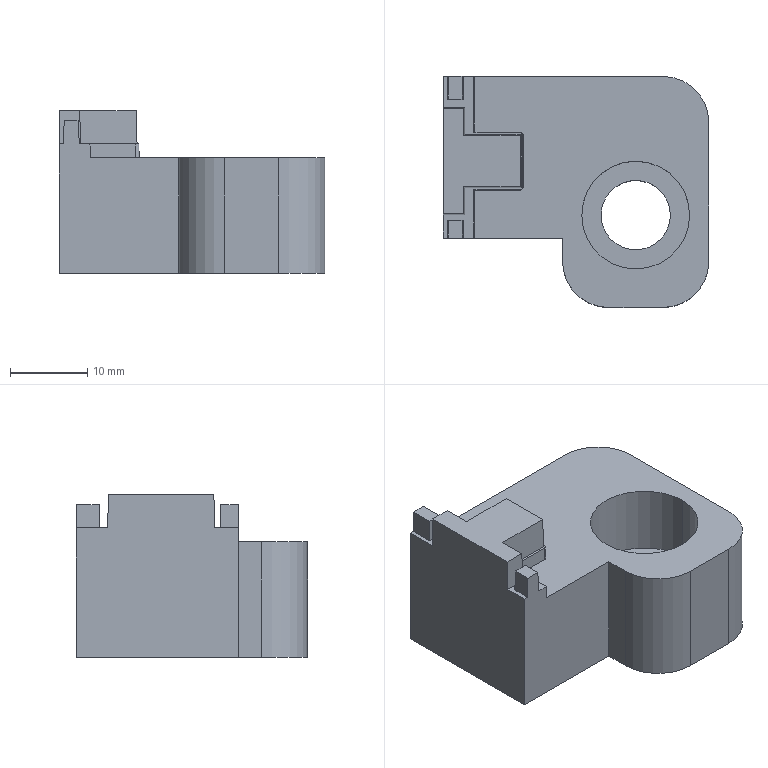Part | Creo | 1 solid | 175 faces | box 34.5 x 30 x 21.126 mm | volume 11962 mm3 | other 107 | plane 58 | cylinder 8 | cone 2 | commonest cylinder face diameters 12 x3 9 x2 14 x2 30.388 x1